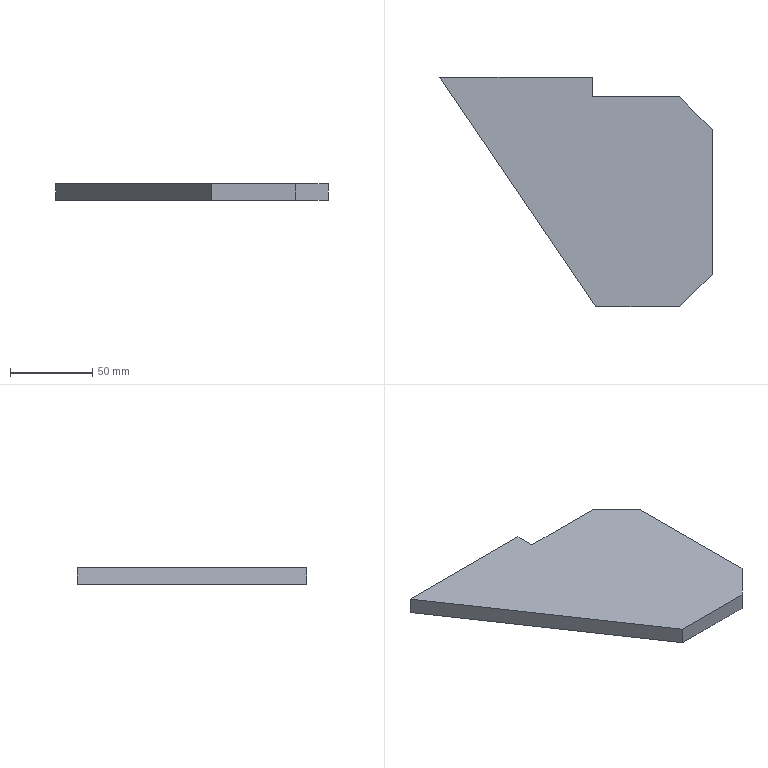Part | STEP file | 08 Rib plate | 1 solid | 10 faces | box 166 x 140 x 10 mm | volume 153140 mm3 | plane 10
STEP:
#1=CARTESIAN_POINT('',(0.,0.,0.));
#2=DIRECTION('',(0.,0.,1.));
#3=DIRECTION('',(1.,0.,0.));
#4=AXIS2_PLACEMENT_3D('',#1,#2,#3);
#5=CARTESIAN_POINT('',(0.,0.,0.));
#6=VERTEX_POINT('',#5);
#7=CARTESIAN_POINT('',(95.,-140.,0.));
#8=VERTEX_POINT('',#7);
#9=CARTESIAN_POINT('',(0.,0.,0.));
#10=DIRECTION('',(0.5615,-0.8275,0.));
#11=VECTOR('',#10,1.);
#12=LINE('',#9,#11);
#13=CARTESIAN_POINT('',(0.,0.,10.));
#14=DIRECTION('',(0.8275,0.5615,0.));
#15=DIRECTION('',(-0.5615,0.8275,0.));
#16=AXIS2_PLACEMENT_3D('',#13,#14,#15);
#17=PLANE('',#16);
#18=CARTESIAN_POINT('',(0.,-10.));
#19=DIRECTION('',(-1.,0.));
#20=VECTOR('',#19,1.);
#21=LINE('',#18,#20);
#22=(GEOMETRIC_REPRESENTATION_CONTEXT(2)PARAMETRIC_REPRESENTATION_CONTEXT()REPRESENTATION_CONTEXT('',''));
#23=DEFINITIONAL_REPRESENTATION('',(#21),#22);
#24=PCURVE('',#17,#23);
#25=CARTESIAN_POINT('',(0.,0.,0.));
#26=DIRECTION('',(0.,0.,-1.));
#27=DIRECTION('',(-1.,0.,0.));
#28=AXIS2_PLACEMENT_3D('',#25,#26,#27);
#29=PLANE('',#28);
#30=CARTESIAN_POINT('',(0.,0.));
#31=DIRECTION('',(-0.5615,-0.8275));
#32=VECTOR('',#31,1.);
#33=LINE('',#30,#32);
#34=(GEOMETRIC_REPRESENTATION_CONTEXT(2)PARAMETRIC_REPRESENTATION_CONTEXT()REPRESENTATION_CONTEXT('',''));
#35=DEFINITIONAL_REPRESENTATION('',(#33),#34);
#36=PCURVE('',#29,#35);
#37=SURFACE_CURVE('',#12,(#24,#36),.PCURVE_S1.);
#38=EDGE_CURVE('',#6,#8,#37,.T.);
#39=ORIENTED_EDGE('',*,*,#38,.T.);
#40=CARTESIAN_POINT('',(95.,-140.,10.));
#41=VERTEX_POINT('',#40);
#42=CARTESIAN_POINT('',(95.,-140.,10.));
#43=DIRECTION('',(0.,0.,-1.));
#44=VECTOR('',#43,1.);
#45=LINE('',#42,#44);
#46=CARTESIAN_POINT('',(-169.189,0.));
#47=DIRECTION('',(0.,-1.));
#48=VECTOR('',#47,1.);
#49=LINE('',#46,#48);
#50=(GEOMETRIC_REPRESENTATION_CONTEXT(2)PARAMETRIC_REPRESENTATION_CONTEXT()REPRESENTATION_CONTEXT('',''));
#51=DEFINITIONAL_REPRESENTATION('',(#49),#50);
#52=PCURVE('',#17,#51);
#53=CARTESIAN_POINT('',(95.,-140.,10.));
#54=DIRECTION('',(0.,1.,0.));
#55=DIRECTION('',(0.,0.,1.));
#56=AXIS2_PLACEMENT_3D('',#53,#54,#55);
#57=PLANE('',#56);
#58=CARTESIAN_POINT('',(0.,0.));
#59=DIRECTION('',(-1.,0.));
#60=VECTOR('',#59,1.);
#61=LINE('',#58,#60);
#62=(GEOMETRIC_REPRESENTATION_CONTEXT(2)PARAMETRIC_REPRESENTATION_CONTEXT()REPRESENTATION_CONTEXT('',''));
#63=DEFINITIONAL_REPRESENTATION('',(#61),#62);
#64=PCURVE('',#57,#63);
#65=SURFACE_CURVE('',#45,(#52,#64),.PCURVE_S1.);
#66=EDGE_CURVE('',#41,#8,#65,.T.);
#67=ORIENTED_EDGE('',*,*,#66,.F.);
#68=CARTESIAN_POINT('',(0.,0.,10.));
#69=VERTEX_POINT('',#68);
#70=CARTESIAN_POINT('',(0.,0.,10.));
#71=DIRECTION('',(0.5615,-0.8275,0.));
#72=VECTOR('',#71,1.);
#73=LINE('',#70,#72);
#74=CARTESIAN_POINT('',(0.,0.));
#75=DIRECTION('',(-1.,0.));
#76=VECTOR('',#75,1.);
#77=LINE('',#74,#76);
#78=(GEOMETRIC_REPRESENTATION_CONTEXT(2)PARAMETRIC_REPRESENTATION_CONTEXT()REPRESENTATION_CONTEXT('',''));
#79=DEFINITIONAL_REPRESENTATION('',(#77),#78);
#80=PCURVE('',#17,#79);
#81=CARTESIAN_POINT('',(0.,0.,10.));
#82=DIRECTION('',(0.,0.,-1.));
#83=DIRECTION('',(-1.,0.,0.));
#84=AXIS2_PLACEMENT_3D('',#81,#82,#83);
#85=PLANE('',#84);
#86=CARTESIAN_POINT('',(0.,0.));
#87=DIRECTION('',(-0.5615,-0.8275));
#88=VECTOR('',#87,1.);
#89=LINE('',#86,#88);
#90=(GEOMETRIC_REPRESENTATION_CONTEXT(2)PARAMETRIC_REPRESENTATION_CONTEXT()REPRESENTATION_CONTEXT('',''));
#91=DEFINITIONAL_REPRESENTATION('',(#89),#90);
#92=PCURVE('',#85,#91);
#93=SURFACE_CURVE('',#73,(#80,#92),.PCURVE_S1.);
#94=EDGE_CURVE('',#69,#41,#93,.T.);
#95=ORIENTED_EDGE('',*,*,#94,.F.);
#96=CARTESIAN_POINT('',(0.,0.,10.));
#97=DIRECTION('',(0.,0.,-1.));
#98=VECTOR('',#97,1.);
#99=LINE('',#96,#98);
#100=CARTESIAN_POINT('',(0.,0.));
#101=DIRECTION('',(0.,-1.));
#102=VECTOR('',#101,1.);
#103=LINE('',#100,#102);
#104=(GEOMETRIC_REPRESENTATION_CONTEXT(2)PARAMETRIC_REPRESENTATION_CONTEXT()REPRESENTATION_CONTEXT('',''));
#105=DEFINITIONAL_REPRESENTATION('',(#103),#104);
#106=PCURVE('',#17,#105);
#107=CARTESIAN_POINT('',(0.,0.,10.));
#108=DIRECTION('',(0.,-1.,0.));
#109=DIRECTION('',(0.,0.,-1.));
#110=AXIS2_PLACEMENT_3D('',#107,#108,#109);
#111=PLANE('',#110);
#112=CARTESIAN_POINT('',(0.,0.));
#113=DIRECTION('',(1.,0.));
#114=VECTOR('',#113,1.);
#115=LINE('',#112,#114);
#116=(GEOMETRIC_REPRESENTATION_CONTEXT(2)PARAMETRIC_REPRESENTATION_CONTEXT()REPRESENTATION_CONTEXT('',''));
#117=DEFINITIONAL_REPRESENTATION('',(#115),#116);
#118=PCURVE('',#111,#117);
#119=SURFACE_CURVE('',#99,(#106,#118),.PCURVE_S1.);
#120=EDGE_CURVE('',#69,#6,#119,.T.);
#121=ORIENTED_EDGE('',*,*,#120,.T.);
#122=EDGE_LOOP('',(#39,#67,#95,#121));
#123=FACE_BOUND('',#122,.T.);
#124=ADVANCED_FACE('',(#123),#17,.F.);
#125=CARTESIAN_POINT('',(146.,-140.,0.));
#126=VERTEX_POINT('',#125);
#127=CARTESIAN_POINT('',(95.,-140.,0.));
#128=DIRECTION('',(1.,0.,0.));
#129=VECTOR('',#128,1.);
#130=LINE('',#127,#129);
#131=CARTESIAN_POINT('',(-10.,0.));
#132=DIRECTION('',(0.,1.));
#133=VECTOR('',#132,1.);
#134=LINE('',#131,#133);
#135=(GEOMETRIC_REPRESENTATION_CONTEXT(2)PARAMETRIC_REPRESENTATION_CONTEXT()REPRESENTATION_CONTEXT('',''));
#136=DEFINITIONAL_REPRESENTATION('',(#134),#135);
#137=PCURVE('',#57,#136);
#138=CARTESIAN_POINT('',(-95.,-140.));
#139=DIRECTION('',(-1.,0.));
#140=VECTOR('',#139,1.);
#141=LINE('',#138,#140);
#142=(GEOMETRIC_REPRESENTATION_CONTEXT(2)PARAMETRIC_REPRESENTATION_CONTEXT()REPRESENTATION_CONTEXT('',''));
#143=DEFINITIONAL_REPRESENTATION('',(#141),#142);
#144=PCURVE('',#29,#143);
#145=SURFACE_CURVE('',#130,(#137,#144),.PCURVE_S1.);
#146=EDGE_CURVE('',#8,#126,#145,.T.);
#147=ORIENTED_EDGE('',*,*,#146,.T.);
#148=CARTESIAN_POINT('',(146.,-140.,10.));
#149=VERTEX_POINT('',#148);
#150=CARTESIAN_POINT('',(146.,-140.,10.));
#151=DIRECTION('',(0.,0.,-1.));
#152=VECTOR('',#151,1.);
#153=LINE('',#150,#152);
#154=CARTESIAN_POINT('',(0.,51.));
#155=DIRECTION('',(-1.,0.));
#156=VECTOR('',#155,1.);
#157=LINE('',#154,#156);
#158=(GEOMETRIC_REPRESENTATION_CONTEXT(2)PARAMETRIC_REPRESENTATION_CONTEXT()REPRESENTATION_CONTEXT('',''));
#159=DEFINITIONAL_REPRESENTATION('',(#157),#158);
#160=PCURVE('',#57,#159);
#161=CARTESIAN_POINT('',(166.,-120.,10.));
#162=DIRECTION('',(-0.7071,0.7071,0.));
#163=DIRECTION('',(-0.7071,-0.7071,0.));
#164=AXIS2_PLACEMENT_3D('',#161,#162,#163);
#165=PLANE('',#164);
#166=CARTESIAN_POINT('',(28.284,0.));
#167=DIRECTION('',(0.,-1.));
#168=VECTOR('',#167,1.);
#169=LINE('',#166,#168);
#170=(GEOMETRIC_REPRESENTATION_CONTEXT(2)PARAMETRIC_REPRESENTATION_CONTEXT()REPRESENTATION_CONTEXT('',''));
#171=DEFINITIONAL_REPRESENTATION('',(#169),#170);
#172=PCURVE('',#165,#171);
#173=SURFACE_CURVE('',#153,(#160,#172),.PCURVE_S1.);
#174=EDGE_CURVE('',#149,#126,#173,.T.);
#175=ORIENTED_EDGE('',*,*,#174,.F.);
#176=CARTESIAN_POINT('',(95.,-140.,10.));
#177=DIRECTION('',(1.,0.,0.));
#178=VECTOR('',#177,1.);
#179=LINE('',#176,#178);
#180=CARTESIAN_POINT('',(0.,0.));
#181=DIRECTION('',(0.,1.));
#182=VECTOR('',#181,1.);
#183=LINE('',#180,#182);
#184=(GEOMETRIC_REPRESENTATION_CONTEXT(2)PARAMETRIC_REPRESENTATION_CONTEXT()REPRESENTATION_CONTEXT('',''));
#185=DEFINITIONAL_REPRESENTATION('',(#183),#184);
#186=PCURVE('',#57,#185);
#187=CARTESIAN_POINT('',(-95.,-140.));
#188=DIRECTION('',(-1.,0.));
#189=VECTOR('',#188,1.);
#190=LINE('',#187,#189);
#191=(GEOMETRIC_REPRESENTATION_CONTEXT(2)PARAMETRIC_REPRESENTATION_CONTEXT()REPRESENTATION_CONTEXT('',''));
#192=DEFINITIONAL_REPRESENTATION('',(#190),#191);
#193=PCURVE('',#85,#192);
#194=SURFACE_CURVE('',#179,(#186,#193),.PCURVE_S1.);
#195=EDGE_CURVE('',#41,#149,#194,.T.);
#196=ORIENTED_EDGE('',*,*,#195,.F.);
#197=ORIENTED_EDGE('',*,*,#66,.T.);
#198=EDGE_LOOP('',(#147,#175,#196,#197));
#199=FACE_BOUND('',#198,.T.);
#200=ADVANCED_FACE('',(#199),#57,.F.);
#201=CARTESIAN_POINT('',(166.,-120.,0.));
#202=VERTEX_POINT('',#201);
#203=CARTESIAN_POINT('',(166.,-120.,0.));
#204=DIRECTION('',(0.7071,0.7071,0.));
#205=VECTOR('',#204,1.);
#206=LINE('',#203,#205);
#207=CARTESIAN_POINT('',(0.,-10.));
#208=DIRECTION('',(-1.,0.));
#209=VECTOR('',#208,1.);
#210=LINE('',#207,#209);
#211=(GEOMETRIC_REPRESENTATION_CONTEXT(2)PARAMETRIC_REPRESENTATION_CONTEXT()REPRESENTATION_CONTEXT('',''));
#212=DEFINITIONAL_REPRESENTATION('',(#210),#211);
#213=PCURVE('',#165,#212);
#214=CARTESIAN_POINT('',(-166.,-120.));
#215=DIRECTION('',(-0.7071,0.7071));
#216=VECTOR('',#215,1.);
#217=LINE('',#214,#216);
#218=(GEOMETRIC_REPRESENTATION_CONTEXT(2)PARAMETRIC_REPRESENTATION_CONTEXT()REPRESENTATION_CONTEXT('',''));
#219=DEFINITIONAL_REPRESENTATION('',(#217),#218);
#220=PCURVE('',#29,#219);
#221=SURFACE_CURVE('',#206,(#213,#220),.PCURVE_S1.);
#222=EDGE_CURVE('',#126,#202,#221,.T.);
#223=ORIENTED_EDGE('',*,*,#222,.T.);
#224=CARTESIAN_POINT('',(166.,-120.,10.));
#225=VERTEX_POINT('',#224);
#226=CARTESIAN_POINT('',(166.,-120.,10.));
#227=DIRECTION('',(0.,0.,-1.));
#228=VECTOR('',#227,1.);
#229=LINE('',#226,#228);
#230=CARTESIAN_POINT('',(0.,0.));
#231=DIRECTION('',(0.,-1.));
#232=VECTOR('',#231,1.);
#233=LINE('',#230,#232);
#234=(GEOMETRIC_REPRESENTATION_CONTEXT(2)PARAMETRIC_REPRESENTATION_CONTEXT()REPRESENTATION_CONTEXT('',''));
#235=DEFINITIONAL_REPRESENTATION('',(#233),#234);
#236=PCURVE('',#165,#235);
#237=CARTESIAN_POINT('',(166.,-32.,10.));
#238=DIRECTION('',(-1.,0.,0.));
#239=DIRECTION('',(0.,-1.,0.));
#240=AXIS2_PLACEMENT_3D('',#237,#238,#239);
#241=PLANE('',#240);
#242=CARTESIAN_POINT('',(88.,0.));
#243=DIRECTION('',(0.,-1.));
#244=VECTOR('',#243,1.);
#245=LINE('',#242,#244);
#246=(GEOMETRIC_REPRESENTATION_CONTEXT(2)PARAMETRIC_REPRESENTATION_CONTEXT()REPRESENTATION_CONTEXT('',''));
#247=DEFINITIONAL_REPRESENTATION('',(#245),#246);
#248=PCURVE('',#241,#247);
#249=SURFACE_CURVE('',#229,(#236,#248),.PCURVE_S1.);
#250=EDGE_CURVE('',#225,#202,#249,.T.);
#251=ORIENTED_EDGE('',*,*,#250,.F.);
#252=CARTESIAN_POINT('',(166.,-120.,10.));
#253=DIRECTION('',(0.7071,0.7071,0.));
#254=VECTOR('',#253,1.);
#255=LINE('',#252,#254);
#256=CARTESIAN_POINT('',(0.,0.));
#257=DIRECTION('',(-1.,0.));
#258=VECTOR('',#257,1.);
#259=LINE('',#256,#258);
#260=(GEOMETRIC_REPRESENTATION_CONTEXT(2)PARAMETRIC_REPRESENTATION_CONTEXT()REPRESENTATION_CONTEXT('',''));
#261=DEFINITIONAL_REPRESENTATION('',(#259),#260);
#262=PCURVE('',#165,#261);
#263=CARTESIAN_POINT('',(-166.,-120.));
#264=DIRECTION('',(-0.7071,0.7071));
#265=VECTOR('',#264,1.);
#266=LINE('',#263,#265);
#267=(GEOMETRIC_REPRESENTATION_CONTEXT(2)PARAMETRIC_REPRESENTATION_CONTEXT()REPRESENTATION_CONTEXT('',''));
#268=DEFINITIONAL_REPRESENTATION('',(#266),#267);
#269=PCURVE('',#85,#268);
#270=SURFACE_CURVE('',#255,(#262,#269),.PCURVE_S1.);
#271=EDGE_CURVE('',#149,#225,#270,.T.);
#272=ORIENTED_EDGE('',*,*,#271,.F.);
#273=ORIENTED_EDGE('',*,*,#174,.T.);
#274=EDGE_LOOP('',(#223,#251,#272,#273));
#275=FACE_BOUND('',#274,.T.);
#276=ADVANCED_FACE('',(#275),#165,.F.);
#277=CARTESIAN_POINT('',(166.,-32.,0.));
#278=VERTEX_POINT('',#277);
#279=CARTESIAN_POINT('',(166.,-32.,0.));
#280=DIRECTION('',(0.,1.,0.));
#281=VECTOR('',#280,1.);
#282=LINE('',#279,#281);
#283=CARTESIAN_POINT('',(0.,-10.));
#284=DIRECTION('',(-1.,0.));
#285=VECTOR('',#284,1.);
#286=LINE('',#283,#285);
#287=(GEOMETRIC_REPRESENTATION_CONTEXT(2)PARAMETRIC_REPRESENTATION_CONTEXT()REPRESENTATION_CONTEXT('',''));
#288=DEFINITIONAL_REPRESENTATION('',(#286),#287);
#289=PCURVE('',#241,#288);
#290=CARTESIAN_POINT('',(-166.,-32.));
#291=DIRECTION('',(0.,1.));
#292=VECTOR('',#291,1.);
#293=LINE('',#290,#292);
#294=(GEOMETRIC_REPRESENTATION_CONTEXT(2)PARAMETRIC_REPRESENTATION_CONTEXT()REPRESENTATION_CONTEXT('',''));
#295=DEFINITIONAL_REPRESENTATION('',(#293),#294);
#296=PCURVE('',#29,#295);
#297=SURFACE_CURVE('',#282,(#289,#296),.PCURVE_S1.);
#298=EDGE_CURVE('',#202,#278,#297,.T.);
#299=ORIENTED_EDGE('',*,*,#298,.T.);
#300=CARTESIAN_POINT('',(166.,-32.,10.));
#301=VERTEX_POINT('',#300);
#302=CARTESIAN_POINT('',(166.,-32.,10.));
#303=DIRECTION('',(0.,0.,-1.));
#304=VECTOR('',#303,1.);
#305=LINE('',#302,#304);
#306=CARTESIAN_POINT('',(0.,0.));
#307=DIRECTION('',(0.,-1.));
#308=VECTOR('',#307,1.);
#309=LINE('',#306,#308);
#310=(GEOMETRIC_REPRESENTATION_CONTEXT(2)PARAMETRIC_REPRESENTATION_CONTEXT()REPRESENTATION_CONTEXT('',''));
#311=DEFINITIONAL_REPRESENTATION('',(#309),#310);
#312=PCURVE('',#241,#311);
#313=CARTESIAN_POINT('',(146.,-12.,10.));
#314=DIRECTION('',(-0.7071,-0.7071,0.));
#315=DIRECTION('',(0.7071,-0.7071,0.));
#316=AXIS2_PLACEMENT_3D('',#313,#314,#315);
#317=PLANE('',#316);
#318=CARTESIAN_POINT('',(28.284,0.));
#319=DIRECTION('',(0.,-1.));
#320=VECTOR('',#319,1.);
#321=LINE('',#318,#320);
#322=(GEOMETRIC_REPRESENTATION_CONTEXT(2)PARAMETRIC_REPRESENTATION_CONTEXT()REPRESENTATION_CONTEXT('',''));
#323=DEFINITIONAL_REPRESENTATION('',(#321),#322);
#324=PCURVE('',#317,#323);
#325=SURFACE_CURVE('',#305,(#312,#324),.PCURVE_S1.);
#326=EDGE_CURVE('',#301,#278,#325,.T.);
#327=ORIENTED_EDGE('',*,*,#326,.F.);
#328=CARTESIAN_POINT('',(166.,-32.,10.));
#329=DIRECTION('',(0.,1.,0.));
#330=VECTOR('',#329,1.);
#331=LINE('',#328,#330);
#332=CARTESIAN_POINT('',(0.,0.));
#333=DIRECTION('',(-1.,0.));
#334=VECTOR('',#333,1.);
#335=LINE('',#332,#334);
#336=(GEOMETRIC_REPRESENTATION_CONTEXT(2)PARAMETRIC_REPRESENTATION_CONTEXT()REPRESENTATION_CONTEXT('',''));
#337=DEFINITIONAL_REPRESENTATION('',(#335),#336);
#338=PCURVE('',#241,#337);
#339=CARTESIAN_POINT('',(-166.,-32.));
#340=DIRECTION('',(0.,1.));
#341=VECTOR('',#340,1.);
#342=LINE('',#339,#341);
#343=(GEOMETRIC_REPRESENTATION_CONTEXT(2)PARAMETRIC_REPRESENTATION_CONTEXT()REPRESENTATION_CONTEXT('',''));
#344=DEFINITIONAL_REPRESENTATION('',(#342),#343);
#345=PCURVE('',#85,#344);
#346=SURFACE_CURVE('',#331,(#338,#345),.PCURVE_S1.);
#347=EDGE_CURVE('',#225,#301,#346,.T.);
#348=ORIENTED_EDGE('',*,*,#347,.F.);
#349=ORIENTED_EDGE('',*,*,#250,.T.);
#350=EDGE_LOOP('',(#299,#327,#348,#349));
#351=FACE_BOUND('',#350,.T.);
#352=ADVANCED_FACE('',(#351),#241,.F.);
#353=CARTESIAN_POINT('',(146.,-12.,0.));
#354=VERTEX_POINT('',#353);
#355=CARTESIAN_POINT('',(146.,-12.,0.));
#356=DIRECTION('',(-0.7071,0.7071,0.));
#357=VECTOR('',#356,1.);
#358=LINE('',#355,#357);
#359=CARTESIAN_POINT('',(0.,-10.));
#360=DIRECTION('',(-1.,0.));
#361=VECTOR('',#360,1.);
#362=LINE('',#359,#361);
#363=(GEOMETRIC_REPRESENTATION_CONTEXT(2)PARAMETRIC_REPRESENTATION_CONTEXT()REPRESENTATION_CONTEXT('',''));
#364=DEFINITIONAL_REPRESENTATION('',(#362),#363);
#365=PCURVE('',#317,#364);
#366=CARTESIAN_POINT('',(-146.,-12.));
#367=DIRECTION('',(0.7071,0.7071));
#368=VECTOR('',#367,1.);
#369=LINE('',#366,#368);
#370=(GEOMETRIC_REPRESENTATION_CONTEXT(2)PARAMETRIC_REPRESENTATION_CONTEXT()REPRESENTATION_CONTEXT('',''));
#371=DEFINITIONAL_REPRESENTATION('',(#369),#370);
#372=PCURVE('',#29,#371);
#373=SURFACE_CURVE('',#358,(#365,#372),.PCURVE_S1.);
#374=EDGE_CURVE('',#278,#354,#373,.T.);
#375=ORIENTED_EDGE('',*,*,#374,.T.);
#376=CARTESIAN_POINT('',(146.,-12.,10.));
#377=VERTEX_POINT('',#376);
#378=CARTESIAN_POINT('',(146.,-12.,10.));
#379=DIRECTION('',(0.,0.,-1.));
#380=VECTOR('',#379,1.);
#381=LINE('',#378,#380);
#382=CARTESIAN_POINT('',(0.,0.));
#383=DIRECTION('',(0.,-1.));
#384=VECTOR('',#383,1.);
#385=LINE('',#382,#384);
#386=(GEOMETRIC_REPRESENTATION_CONTEXT(2)PARAMETRIC_REPRESENTATION_CONTEXT()REPRESENTATION_CONTEXT('',''));
#387=DEFINITIONAL_REPRESENTATION('',(#385),#386);
#388=PCURVE('',#317,#387);
#389=CARTESIAN_POINT('',(93.,-12.,10.));
#390=DIRECTION('',(0.,-1.,0.));
#391=DIRECTION('',(1.,0.,0.));
#392=AXIS2_PLACEMENT_3D('',#389,#390,#391);
#393=PLANE('',#392);
#394=CARTESIAN_POINT('',(53.,0.));
#395=DIRECTION('',(0.,-1.));
#396=VECTOR('',#395,1.);
#397=LINE('',#394,#396);
#398=(GEOMETRIC_REPRESENTATION_CONTEXT(2)PARAMETRIC_REPRESENTATION_CONTEXT()REPRESENTATION_CONTEXT('',''));
#399=DEFINITIONAL_REPRESENTATION('',(#397),#398);
#400=PCURVE('',#393,#399);
#401=SURFACE_CURVE('',#381,(#388,#400),.PCURVE_S1.);
#402=EDGE_CURVE('',#377,#354,#401,.T.);
#403=ORIENTED_EDGE('',*,*,#402,.F.);
#404=CARTESIAN_POINT('',(146.,-12.,10.));
#405=DIRECTION('',(-0.7071,0.7071,0.));
#406=VECTOR('',#405,1.);
#407=LINE('',#404,#406);
#408=CARTESIAN_POINT('',(0.,0.));
#409=DIRECTION('',(-1.,0.));
#410=VECTOR('',#409,1.);
#411=LINE('',#408,#410);
#412=(GEOMETRIC_REPRESENTATION_CONTEXT(2)PARAMETRIC_REPRESENTATION_CONTEXT()REPRESENTATION_CONTEXT('',''));
#413=DEFINITIONAL_REPRESENTATION('',(#411),#412);
#414=PCURVE('',#317,#413);
#415=CARTESIAN_POINT('',(-146.,-12.));
#416=DIRECTION('',(0.7071,0.7071));
#417=VECTOR('',#416,1.);
#418=LINE('',#415,#417);
#419=(GEOMETRIC_REPRESENTATION_CONTEXT(2)PARAMETRIC_REPRESENTATION_CONTEXT()REPRESENTATION_CONTEXT('',''));
#420=DEFINITIONAL_REPRESENTATION('',(#418),#419);
#421=PCURVE('',#85,#420);
#422=SURFACE_CURVE('',#407,(#414,#421),.PCURVE_S1.);
#423=EDGE_CURVE('',#301,#377,#422,.T.);
#424=ORIENTED_EDGE('',*,*,#423,.F.);
#425=ORIENTED_EDGE('',*,*,#326,.T.);
#426=EDGE_LOOP('',(#375,#403,#424,#425));
#427=FACE_BOUND('',#426,.T.);
#428=ADVANCED_FACE('',(#427),#317,.F.);
#429=CARTESIAN_POINT('',(93.,-12.,0.));
#430=VERTEX_POINT('',#429);
#431=CARTESIAN_POINT('',(93.,-12.,0.));
#432=DIRECTION('',(-1.,0.,0.));
#433=VECTOR('',#432,1.);
#434=LINE('',#431,#433);
#435=CARTESIAN_POINT('',(0.,-10.));
#436=DIRECTION('',(-1.,0.));
#437=VECTOR('',#436,1.);
#438=LINE('',#435,#437);
#439=(GEOMETRIC_REPRESENTATION_CONTEXT(2)PARAMETRIC_REPRESENTATION_CONTEXT()REPRESENTATION_CONTEXT('',''));
#440=DEFINITIONAL_REPRESENTATION('',(#438),#439);
#441=PCURVE('',#393,#440);
#442=CARTESIAN_POINT('',(-93.,-12.));
#443=DIRECTION('',(1.,0.));
#444=VECTOR('',#443,1.);
#445=LINE('',#442,#444);
#446=(GEOMETRIC_REPRESENTATION_CONTEXT(2)PARAMETRIC_REPRESENTATION_CONTEXT()REPRESENTATION_CONTEXT('',''));
#447=DEFINITIONAL_REPRESENTATION('',(#445),#446);
#448=PCURVE('',#29,#447);
#449=SURFACE_CURVE('',#434,(#441,#448),.PCURVE_S1.);
#450=EDGE_CURVE('',#354,#430,#449,.T.);
#451=ORIENTED_EDGE('',*,*,#450,.T.);
#452=CARTESIAN_POINT('',(93.,-12.,10.));
#453=VERTEX_POINT('',#452);
#454=CARTESIAN_POINT('',(93.,-12.,10.));
#455=DIRECTION('',(0.,0.,-1.));
#456=VECTOR('',#455,1.);
#457=LINE('',#454,#456);
#458=CARTESIAN_POINT('',(0.,0.));
#459=DIRECTION('',(0.,-1.));
#460=VECTOR('',#459,1.);
#461=LINE('',#458,#460);
#462=(GEOMETRIC_REPRESENTATION_CONTEXT(2)PARAMETRIC_REPRESENTATION_CONTEXT()REPRESENTATION_CONTEXT('',''));
#463=DEFINITIONAL_REPRESENTATION('',(#461),#462);
#464=PCURVE('',#393,#463);
#465=CARTESIAN_POINT('',(93.,0.,10.));
#466=DIRECTION('',(-1.,0.,0.));
#467=DIRECTION('',(0.,0.,1.));
#468=AXIS2_PLACEMENT_3D('',#465,#466,#467);
#469=PLANE('',#468);
#470=CARTESIAN_POINT('',(0.,-12.));
#471=DIRECTION('',(-1.,0.));
#472=VECTOR('',#471,1.);
#473=LINE('',#470,#472);
#474=(GEOMETRIC_REPRESENTATION_CONTEXT(2)PARAMETRIC_REPRESENTATION_CONTEXT()REPRESENTATION_CONTEXT('',''));
#475=DEFINITIONAL_REPRESENTATION('',(#473),#474);
#476=PCURVE('',#469,#475);
#477=SURFACE_CURVE('',#457,(#464,#476),.PCURVE_S1.);
#478=EDGE_CURVE('',#453,#430,#477,.T.);
#479=ORIENTED_EDGE('',*,*,#478,.F.);
#480=CARTESIAN_POINT('',(93.,-12.,10.));
#481=DIRECTION('',(-1.,0.,0.));
#482=VECTOR('',#481,1.);
#483=LINE('',#480,#482);
#484=CARTESIAN_POINT('',(0.,0.));
#485=DIRECTION('',(-1.,0.));
#486=VECTOR('',#485,1.);
#487=LINE('',#484,#486);
#488=(GEOMETRIC_REPRESENTATION_CONTEXT(2)PARAMETRIC_REPRESENTATION_CONTEXT()REPRESENTATION_CONTEXT('',''));
#489=DEFINITIONAL_REPRESENTATION('',(#487),#488);
#490=PCURVE('',#393,#489);
#491=CARTESIAN_POINT('',(-93.,-12.));
#492=DIRECTION('',(1.,0.));
#493=VECTOR('',#492,1.);
#494=LINE('',#491,#493);
#495=(GEOMETRIC_REPRESENTATION_CONTEXT(2)PARAMETRIC_REPRESENTATION_CONTEXT()REPRESENTATION_CONTEXT('',''));
#496=DEFINITIONAL_REPRESENTATION('',(#494),#495);
#497=PCURVE('',#85,#496);
#498=SURFACE_CURVE('',#483,(#490,#497),.PCURVE_S1.);
#499=EDGE_CURVE('',#377,#453,#498,.T.);
#500=ORIENTED_EDGE('',*,*,#499,.F.);
#501=ORIENTED_EDGE('',*,*,#402,.T.);
#502=EDGE_LOOP('',(#451,#479,#500,#501));
#503=FACE_BOUND('',#502,.T.);
#504=ADVANCED_FACE('',(#503),#393,.F.);
#505=CARTESIAN_POINT('',(93.,0.,0.));
#506=VERTEX_POINT('',#505);
#507=CARTESIAN_POINT('',(93.,0.,0.));
#508=DIRECTION('',(0.,1.,0.));
#509=VECTOR('',#508,1.);
#510=LINE('',#507,#509);
#511=CARTESIAN_POINT('',(-10.,0.));
#512=DIRECTION('',(0.,1.));
#513=VECTOR('',#512,1.);
#514=LINE('',#511,#513);
#515=(GEOMETRIC_REPRESENTATION_CONTEXT(2)PARAMETRIC_REPRESENTATION_CONTEXT()REPRESENTATION_CONTEXT('',''));
#516=DEFINITIONAL_REPRESENTATION('',(#514),#515);
#517=PCURVE('',#469,#516);
#518=CARTESIAN_POINT('',(-93.,0.));
#519=DIRECTION('',(0.,1.));
#520=VECTOR('',#519,1.);
#521=LINE('',#518,#520);
#522=(GEOMETRIC_REPRESENTATION_CONTEXT(2)PARAMETRIC_REPRESENTATION_CONTEXT()REPRESENTATION_CONTEXT('',''));
#523=DEFINITIONAL_REPRESENTATION('',(#521),#522);
#524=PCURVE('',#29,#523);
#525=SURFACE_CURVE('',#510,(#517,#524),.PCURVE_S1.);
#526=EDGE_CURVE('',#430,#506,#525,.T.);
#527=ORIENTED_EDGE('',*,*,#526,.T.);
#528=CARTESIAN_POINT('',(93.,0.,10.));
#529=VERTEX_POINT('',#528);
#530=CARTESIAN_POINT('',(93.,0.,10.));
#531=DIRECTION('',(0.,0.,-1.));
#532=VECTOR('',#531,1.);
#533=LINE('',#530,#532);
#534=CARTESIAN_POINT('',(0.,0.));
#535=DIRECTION('',(-1.,0.));
#536=VECTOR('',#535,1.);
#537=LINE('',#534,#536);
#538=(GEOMETRIC_REPRESENTATION_CONTEXT(2)PARAMETRIC_REPRESENTATION_CONTEXT()REPRESENTATION_CONTEXT('',''));
#539=DEFINITIONAL_REPRESENTATION('',(#537),#538);
#540=PCURVE('',#469,#539);
#541=CARTESIAN_POINT('',(0.,93.));
#542=DIRECTION('',(1.,0.));
#543=VECTOR('',#542,1.);
#544=LINE('',#541,#543);
#545=(GEOMETRIC_REPRESENTATION_CONTEXT(2)PARAMETRIC_REPRESENTATION_CONTEXT()REPRESENTATION_CONTEXT('',''));
#546=DEFINITIONAL_REPRESENTATION('',(#544),#545);
#547=PCURVE('',#111,#546);
#548=SURFACE_CURVE('',#533,(#540,#547),.PCURVE_S1.);
#549=EDGE_CURVE('',#529,#506,#548,.T.);
#550=ORIENTED_EDGE('',*,*,#549,.F.);
#551=CARTESIAN_POINT('',(93.,0.,10.));
#552=DIRECTION('',(0.,1.,0.));
#553=VECTOR('',#552,1.);
#554=LINE('',#551,#553);
#555=CARTESIAN_POINT('',(0.,0.));
#556=DIRECTION('',(0.,1.));
#557=VECTOR('',#556,1.);
#558=LINE('',#555,#557);
#559=(GEOMETRIC_REPRESENTATION_CONTEXT(2)PARAMETRIC_REPRESENTATION_CONTEXT()REPRESENTATION_CONTEXT('',''));
#560=DEFINITIONAL_REPRESENTATION('',(#558),#559);
#561=PCURVE('',#469,#560);
#562=CARTESIAN_POINT('',(-93.,0.));
#563=DIRECTION('',(0.,1.));
#564=VECTOR('',#563,1.);
#565=LINE('',#562,#564);
#566=(GEOMETRIC_REPRESENTATION_CONTEXT(2)PARAMETRIC_REPRESENTATION_CONTEXT()REPRESENTATION_CONTEXT('',''));
#567=DEFINITIONAL_REPRESENTATION('',(#565),#566);
#568=PCURVE('',#85,#567);
#569=SURFACE_CURVE('',#554,(#561,#568),.PCURVE_S1.);
#570=EDGE_CURVE('',#453,#529,#569,.T.);
#571=ORIENTED_EDGE('',*,*,#570,.F.);
#572=ORIENTED_EDGE('',*,*,#478,.T.);
#573=EDGE_LOOP('',(#527,#550,#571,#572));
#574=FACE_BOUND('',#573,.T.);
#575=ADVANCED_FACE('',(#574),#469,.F.);
#576=CARTESIAN_POINT('',(0.,0.,0.));
#577=DIRECTION('',(-1.,0.,0.));
#578=VECTOR('',#577,1.);
#579=LINE('',#576,#578);
#580=CARTESIAN_POINT('',(10.,0.));
#581=DIRECTION('',(0.,-1.));
#582=VECTOR('',#581,1.);
#583=LINE('',#580,#582);
#584=(GEOMETRIC_REPRESENTATION_CONTEXT(2)PARAMETRIC_REPRESENTATION_CONTEXT()REPRESENTATION_CONTEXT('',''));
#585=DEFINITIONAL_REPRESENTATION('',(#583),#584);
#586=PCURVE('',#111,#585);
#587=CARTESIAN_POINT('',(0.,0.));
#588=DIRECTION('',(1.,0.));
#589=VECTOR('',#588,1.);
#590=LINE('',#587,#589);
#591=(GEOMETRIC_REPRESENTATION_CONTEXT(2)PARAMETRIC_REPRESENTATION_CONTEXT()REPRESENTATION_CONTEXT('',''));
#592=DEFINITIONAL_REPRESENTATION('',(#590),#591);
#593=PCURVE('',#29,#592);
#594=SURFACE_CURVE('',#579,(#586,#593),.PCURVE_S1.);
#595=EDGE_CURVE('',#506,#6,#594,.T.);
#596=ORIENTED_EDGE('',*,*,#595,.T.);
#597=ORIENTED_EDGE('',*,*,#120,.F.);
#598=CARTESIAN_POINT('',(0.,0.,10.));
#599=DIRECTION('',(-1.,0.,0.));
#600=VECTOR('',#599,1.);
#601=LINE('',#598,#600);
#602=CARTESIAN_POINT('',(0.,0.));
#603=DIRECTION('',(0.,-1.));
#604=VECTOR('',#603,1.);
#605=LINE('',#602,#604);
#606=(GEOMETRIC_REPRESENTATION_CONTEXT(2)PARAMETRIC_REPRESENTATION_CONTEXT()REPRESENTATION_CONTEXT('',''));
#607=DEFINITIONAL_REPRESENTATION('',(#605),#606);
#608=PCURVE('',#111,#607);
#609=CARTESIAN_POINT('',(0.,0.));
#610=DIRECTION('',(1.,0.));
#611=VECTOR('',#610,1.);
#612=LINE('',#609,#611);
#613=(GEOMETRIC_REPRESENTATION_CONTEXT(2)PARAMETRIC_REPRESENTATION_CONTEXT()REPRESENTATION_CONTEXT('',''));
#614=DEFINITIONAL_REPRESENTATION('',(#612),#613);
#615=PCURVE('',#85,#614);
#616=SURFACE_CURVE('',#601,(#608,#615),.PCURVE_S1.);
#617=EDGE_CURVE('',#529,#69,#616,.T.);
#618=ORIENTED_EDGE('',*,*,#617,.F.);
#619=ORIENTED_EDGE('',*,*,#549,.T.);
#620=EDGE_LOOP('',(#596,#597,#618,#619));
#621=FACE_BOUND('',#620,.T.);
#622=ADVANCED_FACE('',(#621),#111,.F.);
#623=ORIENTED_EDGE('',*,*,#94,.T.);
#624=ORIENTED_EDGE('',*,*,#195,.T.);
#625=ORIENTED_EDGE('',*,*,#271,.T.);
#626=ORIENTED_EDGE('',*,*,#347,.T.);
#627=ORIENTED_EDGE('',*,*,#423,.T.);
#628=ORIENTED_EDGE('',*,*,#499,.T.);
#629=ORIENTED_EDGE('',*,*,#570,.T.);
#630=ORIENTED_EDGE('',*,*,#617,.T.);
#631=EDGE_LOOP('',(#623,#624,#625,#626,#627,#628,#629,#630));
#632=FACE_BOUND('',#631,.T.);
#633=ADVANCED_FACE('',(#632),#85,.F.);
#634=ORIENTED_EDGE('',*,*,#38,.F.);
#635=ORIENTED_EDGE('',*,*,#595,.F.);
#636=ORIENTED_EDGE('',*,*,#526,.F.);
#637=ORIENTED_EDGE('',*,*,#450,.F.);
#638=ORIENTED_EDGE('',*,*,#374,.F.);
#639=ORIENTED_EDGE('',*,*,#298,.F.);
#640=ORIENTED_EDGE('',*,*,#222,.F.);
#641=ORIENTED_EDGE('',*,*,#146,.F.);
#642=EDGE_LOOP('',(#634,#635,#636,#637,#638,#639,#640,#641));
#643=FACE_BOUND('',#642,.T.);
#644=ADVANCED_FACE('',(#643),#29,.T.);
#645=CLOSED_SHELL('',(#124,#200,#276,#352,#428,#504,#575,#622,#633,#644));
#646=MANIFOLD_SOLID_BREP('',#645);
#647=(LENGTH_UNIT()NAMED_UNIT(*)SI_UNIT(.MILLI.,.METRE.));
#648=UNCERTAINTY_MEASURE_WITH_UNIT(LENGTH_MEASURE(0.0000001),#647,'','');
#649=(NAMED_UNIT(*)PLANE_ANGLE_UNIT()SI_UNIT($,.RADIAN.));
#650=(NAMED_UNIT(*)SI_UNIT($,.STERADIAN.)SOLID_ANGLE_UNIT());
#651=(GEOMETRIC_REPRESENTATION_CONTEXT(3)GLOBAL_UNCERTAINTY_ASSIGNED_CONTEXT((#648))GLOBAL_UNIT_ASSIGNED_CONTEXT((#647,#649,#650))REPRESENTATION_CONTEXT('',''));
#652=ADVANCED_BREP_SHAPE_REPRESENTATION('',(#4,#646),#651);